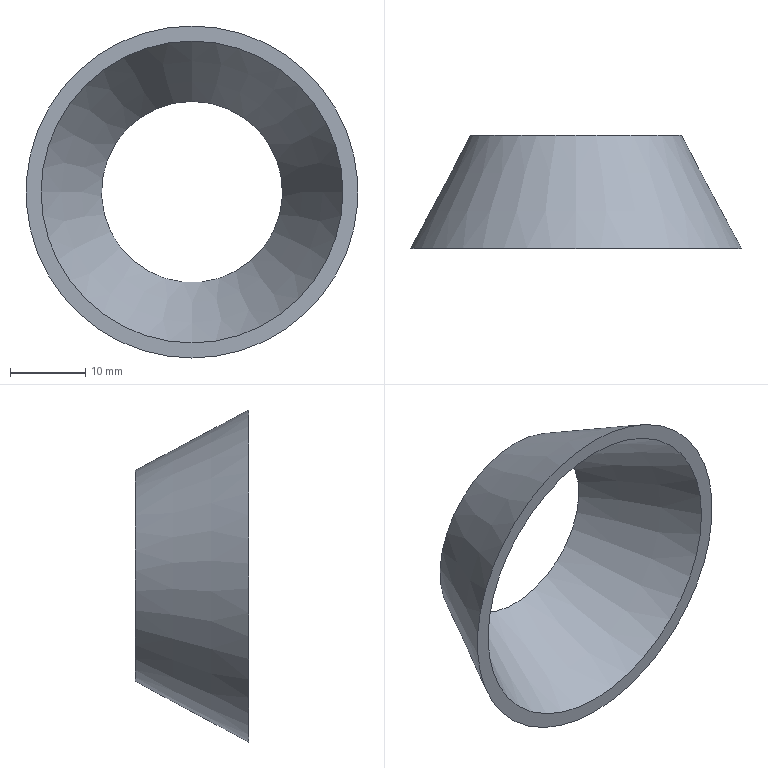Part | NX | features DATUM_CSYS 2, SKETCH 1, SWP104 1 | 1 solid | 4 faces | box 44 x 15 x 44 mm | volume 3204 mm3 | cone 2 | plane 2
STEP:
#1=CARTESIAN_POINT('',(0.,15.,14.));
#2=VERTEX_POINT('',#1);
#3=CARTESIAN_POINT('',(0.,15.,0.));
#4=DIRECTION('',(0.,1.,0.));
#5=DIRECTION('',(0.,0.,1.));
#6=AXIS2_PLACEMENT_3D('',#3,#4,#5);
#7=CIRCLE('',#6,14.);
#8=EDGE_CURVE('',#2,#2,#7,.T.);
#9=ORIENTED_EDGE('',*,*,#8,.F.);
#10=EDGE_LOOP('',(#9));
#11=FACE_BOUND('',#10,.T.);
#12=CARTESIAN_POINT('',(0.,0.,22.));
#13=VERTEX_POINT('',#12);
#14=CARTESIAN_POINT('',(0.,0.,0.));
#15=DIRECTION('',(0.,1.,0.));
#16=DIRECTION('',(0.,0.,1.));
#17=AXIS2_PLACEMENT_3D('',#14,#15,#16);
#18=CIRCLE('',#17,22.);
#19=EDGE_CURVE('',#13,#13,#18,.T.);
#20=ORIENTED_EDGE('',*,*,#19,.T.);
#21=EDGE_LOOP('',(#20));
#22=FACE_BOUND('',#21,.T.);
#23=CARTESIAN_POINT('',(0.,0.,0.));
#24=DIRECTION('',(0.,-1.,0.));
#25=DIRECTION('',(0.,0.,-1.));
#26=AXIS2_PLACEMENT_3D('',#23,#24,#25);
#27=CONICAL_SURFACE('',#26,22.,0.49);
#28=ADVANCED_FACE('',(#11,#22),#27,.T.);
#29=CARTESIAN_POINT('',(0.,15.,12.));
#30=VERTEX_POINT('',#29);
#31=CARTESIAN_POINT('',(0.,15.,0.));
#32=DIRECTION('',(0.,1.,0.));
#33=DIRECTION('',(0.,0.,1.));
#34=AXIS2_PLACEMENT_3D('',#31,#32,#33);
#35=CIRCLE('',#34,12.);
#36=EDGE_CURVE('',#30,#30,#35,.T.);
#37=ORIENTED_EDGE('',*,*,#36,.F.);
#38=EDGE_LOOP('',(#37));
#39=FACE_BOUND('',#38,.T.);
#40=ORIENTED_EDGE('',*,*,#8,.T.);
#41=EDGE_LOOP('',(#40));
#42=FACE_BOUND('',#41,.T.);
#43=CARTESIAN_POINT('',(14.,15.,0.));
#44=DIRECTION('',(0.,-1.,0.));
#45=DIRECTION('',(0.,0.,-1.));
#46=AXIS2_PLACEMENT_3D('',#43,#44,#45);
#47=PLANE('',#46);
#48=ADVANCED_FACE('',(#39,#42),#47,.F.);
#49=CARTESIAN_POINT('',(0.,0.,20.));
#50=VERTEX_POINT('',#49);
#51=CARTESIAN_POINT('',(0.,0.,0.));
#52=DIRECTION('',(0.,1.,0.));
#53=DIRECTION('',(0.,0.,1.));
#54=AXIS2_PLACEMENT_3D('',#51,#52,#53);
#55=CIRCLE('',#54,20.);
#56=EDGE_CURVE('',#50,#50,#55,.T.);
#57=ORIENTED_EDGE('',*,*,#56,.F.);
#58=EDGE_LOOP('',(#57));
#59=FACE_BOUND('',#58,.T.);
#60=ORIENTED_EDGE('',*,*,#36,.T.);
#61=EDGE_LOOP('',(#60));
#62=FACE_BOUND('',#61,.T.);
#63=CARTESIAN_POINT('',(0.,15.,0.));
#64=DIRECTION('',(0.,-1.,0.));
#65=DIRECTION('',(0.,0.,-1.));
#66=AXIS2_PLACEMENT_3D('',#63,#64,#65);
#67=CONICAL_SURFACE('',#66,12.,0.49);
#68=ADVANCED_FACE('',(#59,#62),#67,.F.);
#69=ORIENTED_EDGE('',*,*,#19,.F.);
#70=EDGE_LOOP('',(#69));
#71=FACE_BOUND('',#70,.T.);
#72=ORIENTED_EDGE('',*,*,#56,.T.);
#73=EDGE_LOOP('',(#72));
#74=FACE_BOUND('',#73,.T.);
#75=CARTESIAN_POINT('',(20.,0.,0.));
#76=DIRECTION('',(0.,1.,0.));
#77=DIRECTION('',(0.,0.,1.));
#78=AXIS2_PLACEMENT_3D('',#75,#76,#77);
#79=PLANE('',#78);
#80=ADVANCED_FACE('',(#71,#74),#79,.F.);
#81=CLOSED_SHELL('',(#28,#48,#68,#80));
#82=MANIFOLD_SOLID_BREP('',#81);
#83=(LENGTH_UNIT()NAMED_UNIT(*)SI_UNIT(.MILLI.,.METRE.));
#84=UNCERTAINTY_MEASURE_WITH_UNIT(LENGTH_MEASURE(0.00001),#83,'','');
#85=(NAMED_UNIT(*)PLANE_ANGLE_UNIT()SI_UNIT($,.RADIAN.));
#86=(NAMED_UNIT(*)SI_UNIT($,.STERADIAN.)SOLID_ANGLE_UNIT());
#87=(GEOMETRIC_REPRESENTATION_CONTEXT(3)GLOBAL_UNCERTAINTY_ASSIGNED_CONTEXT((#84))GLOBAL_UNIT_ASSIGNED_CONTEXT((#83,#85,#86))REPRESENTATION_CONTEXT('',''));
#88=ADVANCED_BREP_SHAPE_REPRESENTATION('',(#82),#87);